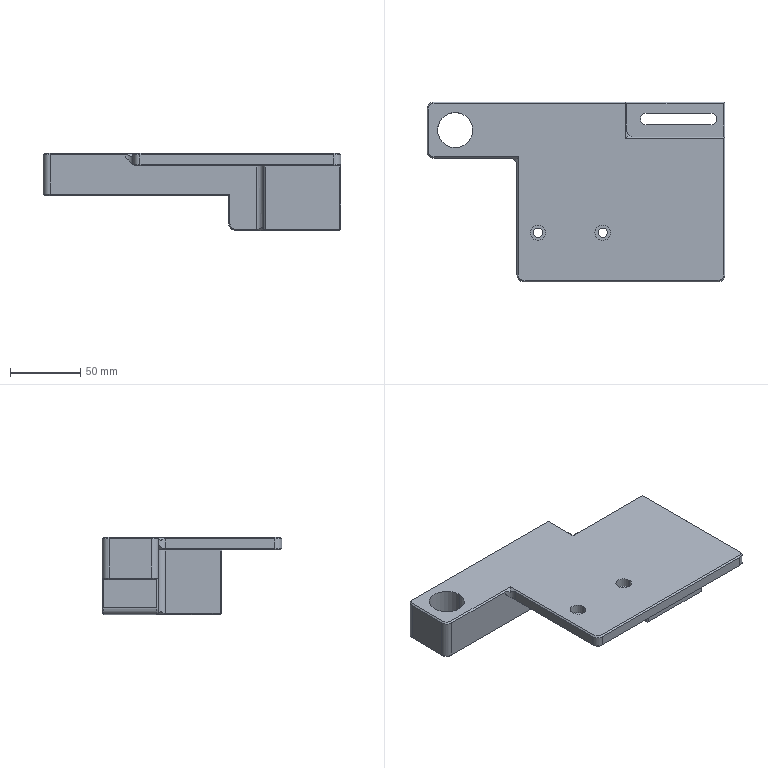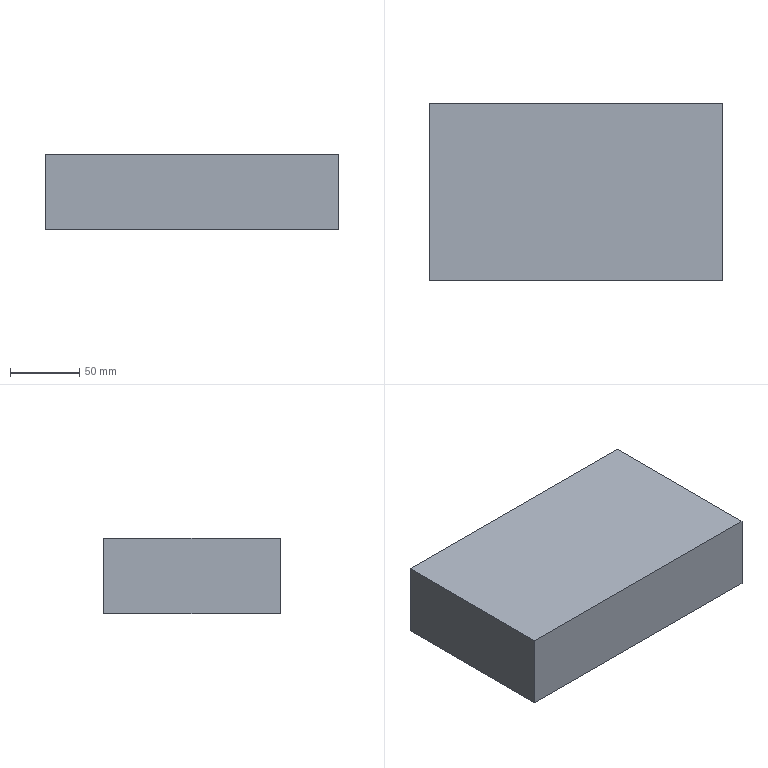CAM job | NX | 3-axis milling, drilling | part box 212 x 128 x 55 mm | stock box 212 x 128 x 55 mm
Tools:
number,name,description,diameter,corner_radius,flute_length,length,flutes
6,D8A45,Milling Tool-5 Parameters,8.0,0.0,4.0,4.0,2
15,6.6ZT,Drilling Tool,6.6,0.0,35.0,50.0,2
17,10.5ZT,Drilling Tool,10.5,0.0,35.0,50.0,2
19,D17R0.8,Milling Tool-5 Parameters,17.0,0.8,50.0,75.0,2
9,D10,Milling Tool-5 Parameters,10.0,0.0,50.0,75.0,2
7,D6,Milling Tool-5 Parameters,6.0,0.0,50.0,75.0,2
21,D50R0.8,Milling Tool-5 Parameters,50.0,0.8,50.0,75.0,2
Operations:
program,operation,operation_type,tool,method,geometry_group,spindle_rpm,surface_speed,feed_per_tooth,feed_cut,feed_plunge,cut_length_mm,path_length_mm,cut_time_min,machine_time_min
1,DRILLING_COPY_2,Operation,D8A45,METHOD,A,3000.0,56.0,0.025,150.0,0.0,12.0,230.007,0.08,0.1018
1,DRILLING_COPY_COPY_COPY_COPY_1_COPY,Operation,6.6ZT,METHOD,A,2000.0,20.0,0.025,100.0,0.0,30.966,171.029,0.3097,0.3237
1,DRILLING_COPY_COPY_COPY_COPY_1_COPY_COPY,Operation,10.5ZT,METHOD,A,1000.0,32.0,0.05,100.0,0.0,37.654,135.309,0.3765,0.3863
1,ZLEVEL_PROFILE,ZLevelMilling,D17R0.8,METHOD,A,2000.0,106.0,0.5,2000.0,1000.0,32827.027,32997.037,16.848,16.865
1,ZLEVEL_PROFILE_COPY,ZLevelMilling,D17R0.8,METHOD,A,2000.0,106.0,0.5,2000.0,1000.0,5639.155,5809.195,3.254,3.271
1,ZLEVEL_PROFILE_COPY_COPY,ZLevelMilling,D17R0.8,METHOD,A,2000.0,106.0,0.5,2000.0,1000.0,1040.886,1120.937,0.6005,0.6085
1,刀补12_COPY,CylinderMilling,D17R0.8,METHOD,A,2000.0,106.0,0.5,2000.0,100.0,2609.914,2700.414,1.305,1.314
1,FLOOR_WALL,VolumeBased25DMillingOperation,D17R0.8,METHOD,A,2000.0,106.0,0.5,2000.0,100.0,34476.9,34610.7,17.238,17.252
1,ZLEVEL_PROFILE_COPY_COPY_COPY,ZLevelMilling,D10,METHOD,A,2000.0,106.0,0.5,2000.0,1000.0,2819.039,4079.399,1.729,1.855
1,FLOOR_WALL_COPY_COPY,VolumeBased25DMillingOperation,D10,METHOD,A,5000.0,157.0,0.1,1000.0,100.0,317.116,800.723,0.3171,0.3655
1,FLOOR_WALL_COPY,VolumeBased25DMillingOperation,D10,METHOD,A,5000.0,157.0,0.1,1000.0,100.0,377.0,509.0,0.377,0.3902
1,HOLE_MILLING,CylinderMilling,D6,METHOD,A,4000.0,75.0,0.1625,1300.0,100.0,2214.867,2392.667,1.704,1.722
1,ZLEVEL_PROFILE_1_COPY_1_COPY_COPY_1_COPY_COPY,ZLevelMilling,D8A45,METHOD,A,6500.0,163.0,0.0769,1000.0,100.0,688.154,752.154,0.6882,0.6946
1,ZLEVEL_PROFILE_1_COPY_1_COPY_COPY_1_COPY_COPY_COPY_1,ZLevelMilling,D8A45,METHOD,A,6500.0,163.0,0.0769,1000.0,100.0,152.368,516.984,0.1524,0.1888
1,ZLEVEL_PROFILE_1_COPY_1_COPY_COPY_1_COPY_COPY_COPY_1_COPY,ZLevelMilling,D8A45,METHOD,A,6500.0,163.0,0.0769,1000.0,100.0,95.005,231.005,0.095,0.1086
1,刀补12,CylinderMilling,D10,METHOD,A,5000.0,157.0,0.1,1000.0,100.0,427.48,516.98,0.4275,0.4364
2,FLOOR_WALL_COPY_1,VolumeBased25DMillingOperation,D50R0.8,METHOD,B,1200.0,188.0,0.5,1200.0,100.0,52843.572,68741.272,44.036,45.626
2,FLOOR_WALL_COPY_1_COPY,VolumeBased25DMillingOperation,D50R0.8,METHOD,B,1200.0,188.0,0.5,1200.0,100.0,19060.517,19170.317,15.884,15.895
2,ZLEVEL_PROFILE_COPY_COPY_COPY_COPY,ZLevelMilling,D17R0.8,METHOD,B,2000.0,106.0,0.5,2000.0,1000.0,6155.954,9636.464,3.429,3.777
2,ZLEVEL_PROFILE_COPY_1,ZLevelMilling,D17R0.8,METHOD,B,6000.0,320.0,0.2083,2500.0,1000.0,5423.673,5483.679,2.178,2.184
2,ZLEVEL_PROFILE_COPY_COPY_COPY_COPY_1,ZLevelMilling,D10,METHOD,B,2000.0,106.0,0.5,2000.0,1000.0,2845.045,4255.285,1.748,1.889
2,FLOOR_WALL_COPY_COPY_COPY,VolumeBased25DMillingOperation,D10,METHOD,B,5000.0,157.0,0.1,1000.0,100.0,121.495,372.859,0.1215,0.1466
2,FLOOR_WALL_COPY_COPY_COPY_COPY,VolumeBased25DMillingOperation,D10,METHOD,B,5000.0,157.0,0.1,1000.0,100.0,629.331,1320.67,0.6293,0.6985
2,FLOOR_WALL_COPY_COPY_1,VolumeBased25DMillingOperation,D10,METHOD,B,5000.0,157.0,0.1,1000.0,100.0,3702.026,4382.84,3.702,3.77
2,ZLEVEL_PROFILE_1,ZLevelMilling,D10,METHOD,B,3000.0,160.0,0.25,1500.0,1000.0,3182.482,3245.482,2.132,2.139
2,ZLEVEL_PROFILE_1_COPY,ZLevelMilling,D6,METHOD,B,4000.0,75.0,0.175,1400.0,1000.0,11907.285,11988.285,8.514,8.522
2,ZLEVEL_PROFILE_1_COPY_1_COPY_COPY_1_COPY_COPY_COPY,ZLevelMilling,D8A45,METHOD,B,6500.0,163.0,0.0769,1000.0,100.0,289.099,353.099,0.2891,0.2955
2,ZLEVEL_PROFILE_1_COPY_1_COPY_COPY_1_COPY_COPY_COPY_COPY_1,ZLevelMilling,D8A45,METHOD,B,6500.0,163.0,0.0769,1000.0,100.0,130.842,192.842,0.1308,0.137
2,ZLEVEL_PROFILE_1_COPY_1_COPY_COPY_1_COPY_COPY_COPY_COPY,ZLevelMilling,D8A45,METHOD,B,6500.0,163.0,0.0769,1000.0,100.0,301.667,413.667,0.3017,0.3129
2,ZLEVEL_PROFILE_1_COPY_1_COPY_COPY_1_COPY_COPY_COPY_COPY_COPY_1,ZLevelMilling,D8A45,METHOD,B,6500.0,163.0,0.0769,1000.0,100.0,73.214,185.214,0.0732,0.0844
2,ZLEVEL_PROFILE_1_COPY_1_COPY_COPY_1_COPY_COPY_COPY_COPY_COPY,ZLevelMilling,D8A45,METHOD,B,6500.0,163.0,0.0769,1000.0,100.0,302.106,886.111,0.3021,0.3605
2,ZLEVEL_PROFILE_1_COPY_1_COPY_COPY_1_COPY_COPY_COPY_COPY_COPY_COPY,ZLevelMilling,D8A45,METHOD,B,6500.0,163.0,0.0769,1000.0,100.0,42.565,392.048,0.0426,0.0775